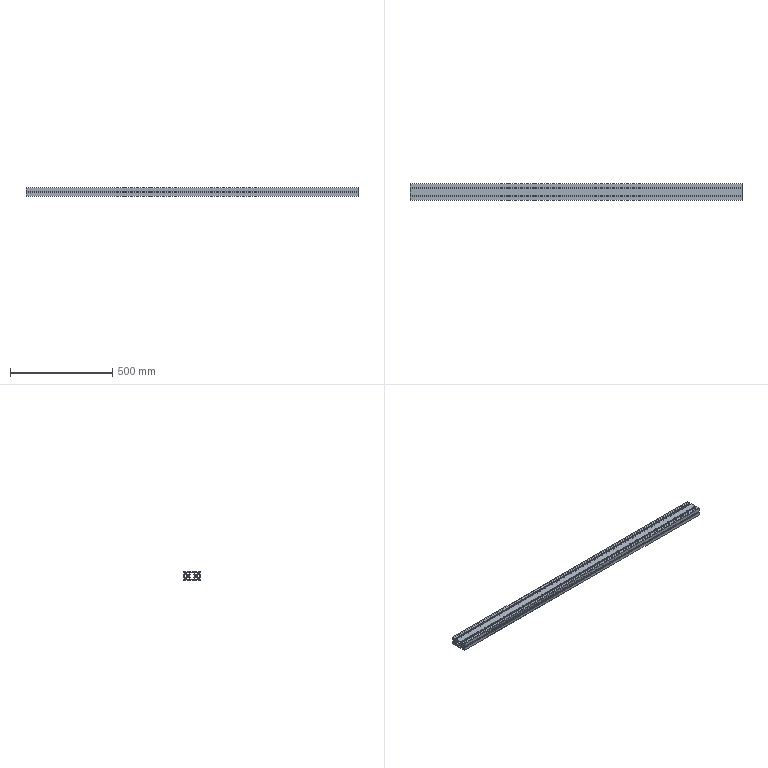Part | SolidWorks | features BaseBody 1 | 1 solid | 90 faces | box 1620 x 80 x 40 mm | volume 1996548 mm3 | plane 66 | cylinder 24 | commonest cylinder face diameters 10 x12 8 x8 6.2 x4